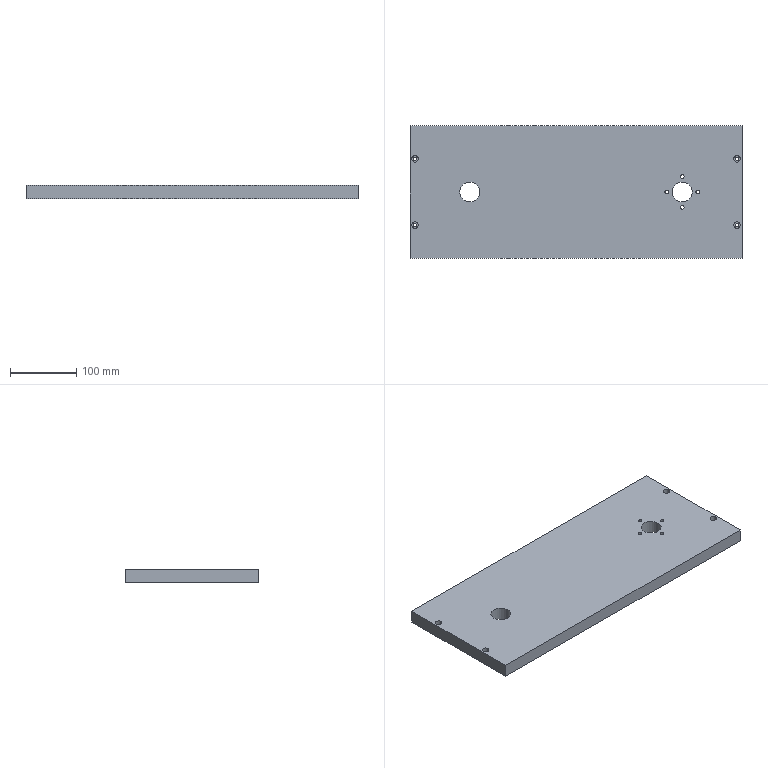Part | NX | features DATUM_CSYS 5, CBORE_HOLE 4, SKETCH 4, EXTRUDE 3, HOLE PACKAGE 1 | 1 solid | 24 faces | box 500 x 200 x 20 mm | volume 1965834 mm3 | cylinder 14 | plane 10 | commonest cylinder face diameters 5.2 x4 5.5 x4 10 x4 30 x2
STEP:
#1=CARTESIAN_POINT('',(183.33,2.75,20.));
#2=VERTEX_POINT('',#1);
#3=CARTESIAN_POINT('',(183.33,0.,20.));
#4=DIRECTION('',(0.,0.,1.));
#5=DIRECTION('',(0.,1.,0.));
#6=AXIS2_PLACEMENT_3D('',#3,#4,#5);
#7=CIRCLE('',#6,2.75);
#8=EDGE_CURVE('',#2,#2,#7,.T.);
#9=ORIENTED_EDGE('',*,*,#8,.F.);
#10=EDGE_LOOP('',(#9));
#11=FACE_BOUND('',#10,.T.);
#12=CARTESIAN_POINT('',(157.25,23.33,20.));
#13=VERTEX_POINT('',#12);
#14=CARTESIAN_POINT('',(160.,23.33,20.));
#15=DIRECTION('',(0.,0.,1.));
#16=DIRECTION('',(-1.,0.,0.));
#17=AXIS2_PLACEMENT_3D('',#14,#15,#16);
#18=CIRCLE('',#17,2.75);
#19=EDGE_CURVE('',#13,#13,#18,.T.);
#20=ORIENTED_EDGE('',*,*,#19,.F.);
#21=EDGE_LOOP('',(#20));
#22=FACE_BOUND('',#21,.T.);
#23=CARTESIAN_POINT('',(162.75,-23.33,20.));
#24=VERTEX_POINT('',#23);
#25=CARTESIAN_POINT('',(160.,-23.33,20.));
#26=DIRECTION('',(0.,0.,1.));
#27=DIRECTION('',(1.,0.,0.));
#28=AXIS2_PLACEMENT_3D('',#25,#26,#27);
#29=CIRCLE('',#28,2.75);
#30=EDGE_CURVE('',#24,#24,#29,.T.);
#31=ORIENTED_EDGE('',*,*,#30,.F.);
#32=EDGE_LOOP('',(#31));
#33=FACE_BOUND('',#32,.T.);
#34=CARTESIAN_POINT('',(136.67,-2.75,20.));
#35=VERTEX_POINT('',#34);
#36=CARTESIAN_POINT('',(136.67,0.,20.));
#37=DIRECTION('',(0.,0.,1.));
#38=DIRECTION('',(0.,-1.,0.));
#39=AXIS2_PLACEMENT_3D('',#36,#37,#38);
#40=CIRCLE('',#39,2.75);
#41=EDGE_CURVE('',#35,#35,#40,.T.);
#42=ORIENTED_EDGE('',*,*,#41,.F.);
#43=EDGE_LOOP('',(#42));
#44=FACE_BOUND('',#43,.T.);
#45=CARTESIAN_POINT('',(237.5,50.,20.));
#46=VERTEX_POINT('',#45);
#47=CARTESIAN_POINT('',(242.5,50.,20.));
#48=DIRECTION('',(0.,0.,-1.));
#49=DIRECTION('',(-1.,0.,0.));
#50=AXIS2_PLACEMENT_3D('',#47,#48,#49);
#51=CIRCLE('',#50,5.);
#52=EDGE_CURVE('',#46,#46,#51,.T.);
#53=ORIENTED_EDGE('',*,*,#52,.T.);
#54=EDGE_LOOP('',(#53));
#55=FACE_BOUND('',#54,.T.);
#56=CARTESIAN_POINT('',(237.5,-50.,20.));
#57=VERTEX_POINT('',#56);
#58=CARTESIAN_POINT('',(242.5,-50.,20.));
#59=DIRECTION('',(0.,0.,-1.));
#60=DIRECTION('',(-1.,0.,0.));
#61=AXIS2_PLACEMENT_3D('',#58,#59,#60);
#62=CIRCLE('',#61,5.);
#63=EDGE_CURVE('',#57,#57,#62,.T.);
#64=ORIENTED_EDGE('',*,*,#63,.T.);
#65=EDGE_LOOP('',(#64));
#66=FACE_BOUND('',#65,.T.);
#67=CARTESIAN_POINT('',(-247.5,50.,20.));
#68=VERTEX_POINT('',#67);
#69=CARTESIAN_POINT('',(-242.5,50.,20.));
#70=DIRECTION('',(0.,0.,-1.));
#71=DIRECTION('',(-1.,0.,0.));
#72=AXIS2_PLACEMENT_3D('',#69,#70,#71);
#73=CIRCLE('',#72,5.);
#74=EDGE_CURVE('',#68,#68,#73,.T.);
#75=ORIENTED_EDGE('',*,*,#74,.T.);
#76=EDGE_LOOP('',(#75));
#77=FACE_BOUND('',#76,.T.);
#78=CARTESIAN_POINT('',(-247.5,-50.,20.));
#79=VERTEX_POINT('',#78);
#80=CARTESIAN_POINT('',(-242.5,-50.,20.));
#81=DIRECTION('',(0.,0.,-1.));
#82=DIRECTION('',(-1.,0.,0.));
#83=AXIS2_PLACEMENT_3D('',#80,#81,#82);
#84=CIRCLE('',#83,5.);
#85=EDGE_CURVE('',#79,#79,#84,.T.);
#86=ORIENTED_EDGE('',*,*,#85,.T.);
#87=EDGE_LOOP('',(#86));
#88=FACE_BOUND('',#87,.T.);
#89=CARTESIAN_POINT('',(-250.,100.,20.));
#90=VERTEX_POINT('',#89);
#91=CARTESIAN_POINT('',(-250.,-100.,20.));
#92=VERTEX_POINT('',#91);
#93=CARTESIAN_POINT('',(-250.,100.,20.));
#94=DIRECTION('',(0.,-1.,0.));
#95=VECTOR('',#94,1000.);
#96=LINE('',#93,#95);
#97=EDGE_CURVE('',#90,#92,#96,.T.);
#98=ORIENTED_EDGE('',*,*,#97,.T.);
#99=CARTESIAN_POINT('',(250.,-100.,20.));
#100=VERTEX_POINT('',#99);
#101=CARTESIAN_POINT('',(-250.,-100.,20.));
#102=DIRECTION('',(1.,0.,0.));
#103=VECTOR('',#102,1000.);
#104=LINE('',#101,#103);
#105=EDGE_CURVE('',#92,#100,#104,.T.);
#106=ORIENTED_EDGE('',*,*,#105,.T.);
#107=CARTESIAN_POINT('',(250.,100.,20.));
#108=VERTEX_POINT('',#107);
#109=CARTESIAN_POINT('',(250.,-100.,20.));
#110=DIRECTION('',(0.,1.,0.));
#111=VECTOR('',#110,1000.);
#112=LINE('',#109,#111);
#113=EDGE_CURVE('',#100,#108,#112,.T.);
#114=ORIENTED_EDGE('',*,*,#113,.T.);
#115=CARTESIAN_POINT('',(250.,100.,20.));
#116=DIRECTION('',(-1.,0.,0.));
#117=VECTOR('',#116,1000.);
#118=LINE('',#115,#117);
#119=EDGE_CURVE('',#108,#90,#118,.T.);
#120=ORIENTED_EDGE('',*,*,#119,.T.);
#121=EDGE_LOOP('',(#98,#106,#114,#120));
#122=FACE_BOUND('',#121,.T.);
#123=CARTESIAN_POINT('',(145.,0.,20.));
#124=VERTEX_POINT('',#123);
#125=CARTESIAN_POINT('',(160.,0.,20.));
#126=DIRECTION('',(0.,0.,-1.));
#127=DIRECTION('',(-1.,0.,0.));
#128=AXIS2_PLACEMENT_3D('',#125,#126,#127);
#129=CIRCLE('',#128,15.);
#130=EDGE_CURVE('',#124,#124,#129,.T.);
#131=ORIENTED_EDGE('',*,*,#130,.T.);
#132=EDGE_LOOP('',(#131));
#133=FACE_BOUND('',#132,.T.);
#134=CARTESIAN_POINT('',(-145.,0.,20.));
#135=VERTEX_POINT('',#134);
#136=CARTESIAN_POINT('',(-160.,0.,20.));
#137=DIRECTION('',(0.,0.,1.));
#138=DIRECTION('',(1.,0.,0.));
#139=AXIS2_PLACEMENT_3D('',#136,#137,#138);
#140=CIRCLE('',#139,15.);
#141=EDGE_CURVE('',#135,#135,#140,.T.);
#142=ORIENTED_EDGE('',*,*,#141,.F.);
#143=EDGE_LOOP('',(#142));
#144=FACE_BOUND('',#143,.T.);
#145=CARTESIAN_POINT('',(0.,0.,20.));
#146=DIRECTION('',(0.,0.,1.));
#147=DIRECTION('',(1.,0.,0.));
#148=AXIS2_PLACEMENT_3D('',#145,#146,#147);
#149=PLANE('',#148);
#150=ADVANCED_FACE('',(#11,#22,#33,#44,#55,#66,#77,#88,#122,#133,#144),#149,.T.);
#151=CARTESIAN_POINT('',(186.08,0.,0.));
#152=VERTEX_POINT('',#151);
#153=CARTESIAN_POINT('',(183.33,0.,0.));
#154=DIRECTION('',(0.,0.,1.));
#155=DIRECTION('',(1.,0.,0.));
#156=AXIS2_PLACEMENT_3D('',#153,#154,#155);
#157=CIRCLE('',#156,2.75);
#158=EDGE_CURVE('',#152,#152,#157,.T.);
#159=ORIENTED_EDGE('',*,*,#158,.T.);
#160=EDGE_LOOP('',(#159));
#161=FACE_BOUND('',#160,.T.);
#162=CARTESIAN_POINT('',(162.75,23.33,0.));
#163=VERTEX_POINT('',#162);
#164=CARTESIAN_POINT('',(160.,23.33,0.));
#165=DIRECTION('',(0.,0.,1.));
#166=DIRECTION('',(1.,0.,0.));
#167=AXIS2_PLACEMENT_3D('',#164,#165,#166);
#168=CIRCLE('',#167,2.75);
#169=EDGE_CURVE('',#163,#163,#168,.T.);
#170=ORIENTED_EDGE('',*,*,#169,.T.);
#171=EDGE_LOOP('',(#170));
#172=FACE_BOUND('',#171,.T.);
#173=CARTESIAN_POINT('',(162.75,-23.33,0.));
#174=VERTEX_POINT('',#173);
#175=CARTESIAN_POINT('',(160.,-23.33,0.));
#176=DIRECTION('',(0.,0.,1.));
#177=DIRECTION('',(1.,0.,0.));
#178=AXIS2_PLACEMENT_3D('',#175,#176,#177);
#179=CIRCLE('',#178,2.75);
#180=EDGE_CURVE('',#174,#174,#179,.T.);
#181=ORIENTED_EDGE('',*,*,#180,.T.);
#182=EDGE_LOOP('',(#181));
#183=FACE_BOUND('',#182,.T.);
#184=CARTESIAN_POINT('',(139.42,0.,0.));
#185=VERTEX_POINT('',#184);
#186=CARTESIAN_POINT('',(136.67,0.,0.));
#187=DIRECTION('',(0.,0.,1.));
#188=DIRECTION('',(1.,0.,0.));
#189=AXIS2_PLACEMENT_3D('',#186,#187,#188);
#190=CIRCLE('',#189,2.75);
#191=EDGE_CURVE('',#185,#185,#190,.T.);
#192=ORIENTED_EDGE('',*,*,#191,.T.);
#193=EDGE_LOOP('',(#192));
#194=FACE_BOUND('',#193,.T.);
#195=CARTESIAN_POINT('',(245.1,50.,0.));
#196=VERTEX_POINT('',#195);
#197=CARTESIAN_POINT('',(242.5,50.,0.));
#198=DIRECTION('',(0.,0.,1.));
#199=DIRECTION('',(1.,0.,0.));
#200=AXIS2_PLACEMENT_3D('',#197,#198,#199);
#201=CIRCLE('',#200,2.6);
#202=EDGE_CURVE('',#196,#196,#201,.T.);
#203=ORIENTED_EDGE('',*,*,#202,.T.);
#204=EDGE_LOOP('',(#203));
#205=FACE_BOUND('',#204,.T.);
#206=CARTESIAN_POINT('',(245.1,-50.,0.));
#207=VERTEX_POINT('',#206);
#208=CARTESIAN_POINT('',(242.5,-50.,0.));
#209=DIRECTION('',(0.,0.,1.));
#210=DIRECTION('',(1.,0.,0.));
#211=AXIS2_PLACEMENT_3D('',#208,#209,#210);
#212=CIRCLE('',#211,2.6);
#213=EDGE_CURVE('',#207,#207,#212,.T.);
#214=ORIENTED_EDGE('',*,*,#213,.T.);
#215=EDGE_LOOP('',(#214));
#216=FACE_BOUND('',#215,.T.);
#217=CARTESIAN_POINT('',(-239.9,50.,0.));
#218=VERTEX_POINT('',#217);
#219=CARTESIAN_POINT('',(-242.5,50.,0.));
#220=DIRECTION('',(0.,0.,1.));
#221=DIRECTION('',(1.,0.,0.));
#222=AXIS2_PLACEMENT_3D('',#219,#220,#221);
#223=CIRCLE('',#222,2.6);
#224=EDGE_CURVE('',#218,#218,#223,.T.);
#225=ORIENTED_EDGE('',*,*,#224,.T.);
#226=EDGE_LOOP('',(#225));
#227=FACE_BOUND('',#226,.T.);
#228=CARTESIAN_POINT('',(-239.9,-50.,0.));
#229=VERTEX_POINT('',#228);
#230=CARTESIAN_POINT('',(-242.5,-50.,0.));
#231=DIRECTION('',(0.,0.,1.));
#232=DIRECTION('',(1.,0.,0.));
#233=AXIS2_PLACEMENT_3D('',#230,#231,#232);
#234=CIRCLE('',#233,2.6);
#235=EDGE_CURVE('',#229,#229,#234,.T.);
#236=ORIENTED_EDGE('',*,*,#235,.T.);
#237=EDGE_LOOP('',(#236));
#238=FACE_BOUND('',#237,.T.);
#239=CARTESIAN_POINT('',(145.,0.,0.));
#240=VERTEX_POINT('',#239);
#241=CARTESIAN_POINT('',(160.,0.,0.));
#242=DIRECTION('',(0.,0.,-1.));
#243=DIRECTION('',(-1.,0.,0.));
#244=AXIS2_PLACEMENT_3D('',#241,#242,#243);
#245=CIRCLE('',#244,15.);
#246=EDGE_CURVE('',#240,#240,#245,.T.);
#247=ORIENTED_EDGE('',*,*,#246,.F.);
#248=EDGE_LOOP('',(#247));
#249=FACE_BOUND('',#248,.T.);
#250=CARTESIAN_POINT('',(-250.,100.,0.));
#251=VERTEX_POINT('',#250);
#252=CARTESIAN_POINT('',(-250.,-100.,0.));
#253=VERTEX_POINT('',#252);
#254=CARTESIAN_POINT('',(-250.,100.,0.));
#255=DIRECTION('',(0.,-1.,0.));
#256=VECTOR('',#255,1000.);
#257=LINE('',#254,#256);
#258=EDGE_CURVE('',#251,#253,#257,.T.);
#259=ORIENTED_EDGE('',*,*,#258,.F.);
#260=CARTESIAN_POINT('',(250.,100.,0.));
#261=VERTEX_POINT('',#260);
#262=CARTESIAN_POINT('',(250.,100.,0.));
#263=DIRECTION('',(-1.,0.,0.));
#264=VECTOR('',#263,1000.);
#265=LINE('',#262,#264);
#266=EDGE_CURVE('',#261,#251,#265,.T.);
#267=ORIENTED_EDGE('',*,*,#266,.F.);
#268=CARTESIAN_POINT('',(250.,-100.,0.));
#269=VERTEX_POINT('',#268);
#270=CARTESIAN_POINT('',(250.,-100.,0.));
#271=DIRECTION('',(0.,1.,0.));
#272=VECTOR('',#271,1000.);
#273=LINE('',#270,#272);
#274=EDGE_CURVE('',#269,#261,#273,.T.);
#275=ORIENTED_EDGE('',*,*,#274,.F.);
#276=CARTESIAN_POINT('',(-250.,-100.,0.));
#277=DIRECTION('',(1.,0.,0.));
#278=VECTOR('',#277,1000.);
#279=LINE('',#276,#278);
#280=EDGE_CURVE('',#253,#269,#279,.T.);
#281=ORIENTED_EDGE('',*,*,#280,.F.);
#282=EDGE_LOOP('',(#259,#267,#275,#281));
#283=FACE_BOUND('',#282,.T.);
#284=CARTESIAN_POINT('',(-145.,0.,0.));
#285=VERTEX_POINT('',#284);
#286=CARTESIAN_POINT('',(-160.,0.,0.));
#287=DIRECTION('',(0.,0.,1.));
#288=DIRECTION('',(1.,0.,0.));
#289=AXIS2_PLACEMENT_3D('',#286,#287,#288);
#290=CIRCLE('',#289,15.);
#291=EDGE_CURVE('',#285,#285,#290,.T.);
#292=ORIENTED_EDGE('',*,*,#291,.T.);
#293=EDGE_LOOP('',(#292));
#294=FACE_BOUND('',#293,.T.);
#295=CARTESIAN_POINT('',(0.,0.,0.));
#296=DIRECTION('',(0.,0.,1.));
#297=DIRECTION('',(1.,0.,0.));
#298=AXIS2_PLACEMENT_3D('',#295,#296,#297);
#299=PLANE('',#298);
#300=ADVANCED_FACE('',(#161,#172,#183,#194,#205,#216,#227,#238,#249,#283,#294),#299,.F.);
#301=ORIENTED_EDGE('',*,*,#258,.T.);
#302=CARTESIAN_POINT('',(-250.,-100.,20.));
#303=DIRECTION('',(0.,0.,-1.));
#304=VECTOR('',#303,1000.);
#305=LINE('',#302,#304);
#306=EDGE_CURVE('',#92,#253,#305,.T.);
#307=ORIENTED_EDGE('',*,*,#306,.F.);
#308=ORIENTED_EDGE('',*,*,#97,.F.);
#309=CARTESIAN_POINT('',(-250.,100.,20.));
#310=DIRECTION('',(0.,0.,-1.));
#311=VECTOR('',#310,1000.);
#312=LINE('',#309,#311);
#313=EDGE_CURVE('',#90,#251,#312,.T.);
#314=ORIENTED_EDGE('',*,*,#313,.T.);
#315=EDGE_LOOP('',(#301,#307,#308,#314));
#316=FACE_BOUND('',#315,.T.);
#317=CARTESIAN_POINT('',(-250.,100.,20.));
#318=DIRECTION('',(1.,0.,0.));
#319=DIRECTION('',(0.,1.,0.));
#320=AXIS2_PLACEMENT_3D('',#317,#318,#319);
#321=PLANE('',#320);
#322=ADVANCED_FACE('',(#316),#321,.F.);
#323=ORIENTED_EDGE('',*,*,#280,.T.);
#324=CARTESIAN_POINT('',(250.,-100.,20.));
#325=DIRECTION('',(0.,0.,-1.));
#326=VECTOR('',#325,1000.);
#327=LINE('',#324,#326);
#328=EDGE_CURVE('',#100,#269,#327,.T.);
#329=ORIENTED_EDGE('',*,*,#328,.F.);
#330=ORIENTED_EDGE('',*,*,#105,.F.);
#331=ORIENTED_EDGE('',*,*,#306,.T.);
#332=EDGE_LOOP('',(#323,#329,#330,#331));
#333=FACE_BOUND('',#332,.T.);
#334=CARTESIAN_POINT('',(-250.,-100.,20.));
#335=DIRECTION('',(0.,1.,0.));
#336=DIRECTION('',(0.,0.,1.));
#337=AXIS2_PLACEMENT_3D('',#334,#335,#336);
#338=PLANE('',#337);
#339=ADVANCED_FACE('',(#333),#338,.F.);
#340=ORIENTED_EDGE('',*,*,#274,.T.);
#341=CARTESIAN_POINT('',(250.,100.,20.));
#342=DIRECTION('',(0.,0.,-1.));
#343=VECTOR('',#342,1000.);
#344=LINE('',#341,#343);
#345=EDGE_CURVE('',#108,#261,#344,.T.);
#346=ORIENTED_EDGE('',*,*,#345,.F.);
#347=ORIENTED_EDGE('',*,*,#113,.F.);
#348=ORIENTED_EDGE('',*,*,#328,.T.);
#349=EDGE_LOOP('',(#340,#346,#347,#348));
#350=FACE_BOUND('',#349,.T.);
#351=CARTESIAN_POINT('',(250.,-100.,20.));
#352=DIRECTION('',(-1.,0.,0.));
#353=DIRECTION('',(0.,-1.,0.));
#354=AXIS2_PLACEMENT_3D('',#351,#352,#353);
#355=PLANE('',#354);
#356=ADVANCED_FACE('',(#350),#355,.F.);
#357=ORIENTED_EDGE('',*,*,#266,.T.);
#358=ORIENTED_EDGE('',*,*,#313,.F.);
#359=ORIENTED_EDGE('',*,*,#119,.F.);
#360=ORIENTED_EDGE('',*,*,#345,.T.);
#361=EDGE_LOOP('',(#357,#358,#359,#360));
#362=FACE_BOUND('',#361,.T.);
#363=CARTESIAN_POINT('',(250.,100.,20.));
#364=DIRECTION('',(0.,-1.,0.));
#365=DIRECTION('',(0.,0.,-1.));
#366=AXIS2_PLACEMENT_3D('',#363,#364,#365);
#367=PLANE('',#366);
#368=ADVANCED_FACE('',(#362),#367,.F.);
#369=ORIENTED_EDGE('',*,*,#130,.F.);
#370=EDGE_LOOP('',(#369));
#371=FACE_BOUND('',#370,.T.);
#372=ORIENTED_EDGE('',*,*,#246,.T.);
#373=EDGE_LOOP('',(#372));
#374=FACE_BOUND('',#373,.T.);
#375=CARTESIAN_POINT('',(160.,0.,20.));
#376=DIRECTION('',(0.,0.,-1.));
#377=DIRECTION('',(-1.,0.,0.));
#378=AXIS2_PLACEMENT_3D('',#375,#376,#377);
#379=CYLINDRICAL_SURFACE('',#378,15.);
#380=ADVANCED_FACE('',(#371,#374),#379,.F.);
#381=ORIENTED_EDGE('',*,*,#141,.T.);
#382=EDGE_LOOP('',(#381));
#383=FACE_BOUND('',#382,.T.);
#384=ORIENTED_EDGE('',*,*,#291,.F.);
#385=EDGE_LOOP('',(#384));
#386=FACE_BOUND('',#385,.T.);
#387=CARTESIAN_POINT('',(-160.,0.,20.));
#388=DIRECTION('',(0.,0.,-1.));
#389=DIRECTION('',(-1.,0.,0.));
#390=AXIS2_PLACEMENT_3D('',#387,#388,#389);
#391=CYLINDRICAL_SURFACE('',#390,15.);
#392=ADVANCED_FACE('',(#383,#386),#391,.F.);
#393=CARTESIAN_POINT('',(-245.1,-50.,10.));
#394=VERTEX_POINT('',#393);
#395=CARTESIAN_POINT('',(-242.5,-50.,10.));
#396=DIRECTION('',(0.,0.,-1.));
#397=DIRECTION('',(-1.,0.,0.));
#398=AXIS2_PLACEMENT_3D('',#395,#396,#397);
#399=CIRCLE('',#398,2.6);
#400=EDGE_CURVE('',#394,#394,#399,.F.);
#401=ORIENTED_EDGE('',*,*,#400,.T.);
#402=EDGE_LOOP('',(#401));
#403=FACE_BOUND('',#402,.T.);
#404=ORIENTED_EDGE('',*,*,#235,.F.);
#405=EDGE_LOOP('',(#404));
#406=FACE_BOUND('',#405,.T.);
#407=CARTESIAN_POINT('',(-242.5,-50.,-30.));
#408=DIRECTION('',(0.,0.,-1.));
#409=DIRECTION('',(-1.,0.,0.));
#410=AXIS2_PLACEMENT_3D('',#407,#408,#409);
#411=CYLINDRICAL_SURFACE('',#410,2.6);
#412=ADVANCED_FACE('',(#403,#406),#411,.F.);
#413=ORIENTED_EDGE('',*,*,#400,.F.);
#414=EDGE_LOOP('',(#413));
#415=FACE_BOUND('',#414,.T.);
#416=CARTESIAN_POINT('',(-247.5,-50.,10.));
#417=VERTEX_POINT('',#416);
#418=CARTESIAN_POINT('',(-242.5,-50.,10.));
#419=DIRECTION('',(0.,0.,-1.));
#420=DIRECTION('',(-1.,0.,0.));
#421=AXIS2_PLACEMENT_3D('',#418,#419,#420);
#422=CIRCLE('',#421,5.);
#423=EDGE_CURVE('',#417,#417,#422,.F.);
#424=ORIENTED_EDGE('',*,*,#423,.T.);
#425=EDGE_LOOP('',(#424));
#426=FACE_BOUND('',#425,.T.);
#427=CARTESIAN_POINT('',(-242.5,-50.,10.));
#428=DIRECTION('',(0.,0.,-1.));
#429=DIRECTION('',(-1.,0.,0.));
#430=AXIS2_PLACEMENT_3D('',#427,#428,#429);
#431=PLANE('',#430);
#432=ADVANCED_FACE('',(#415,#426),#431,.F.);
#433=ORIENTED_EDGE('',*,*,#423,.F.);
#434=EDGE_LOOP('',(#433));
#435=FACE_BOUND('',#434,.T.);
#436=ORIENTED_EDGE('',*,*,#85,.F.);
#437=EDGE_LOOP('',(#436));
#438=FACE_BOUND('',#437,.T.);
#439=CARTESIAN_POINT('',(-242.5,-50.,20.));
#440=DIRECTION('',(0.,0.,-1.));
#441=DIRECTION('',(-1.,0.,0.));
#442=AXIS2_PLACEMENT_3D('',#439,#440,#441);
#443=CYLINDRICAL_SURFACE('',#442,5.);
#444=ADVANCED_FACE('',(#435,#438),#443,.F.);
#445=CARTESIAN_POINT('',(-245.1,50.,10.));
#446=VERTEX_POINT('',#445);
#447=CARTESIAN_POINT('',(-242.5,50.,10.));
#448=DIRECTION('',(0.,0.,-1.));
#449=DIRECTION('',(-1.,0.,0.));
#450=AXIS2_PLACEMENT_3D('',#447,#448,#449);
#451=CIRCLE('',#450,2.6);
#452=EDGE_CURVE('',#446,#446,#451,.F.);
#453=ORIENTED_EDGE('',*,*,#452,.T.);
#454=EDGE_LOOP('',(#453));
#455=FACE_BOUND('',#454,.T.);
#456=ORIENTED_EDGE('',*,*,#224,.F.);
#457=EDGE_LOOP('',(#456));
#458=FACE_BOUND('',#457,.T.);
#459=CARTESIAN_POINT('',(-242.5,50.,-30.));
#460=DIRECTION('',(0.,0.,-1.));
#461=DIRECTION('',(-1.,0.,0.));
#462=AXIS2_PLACEMENT_3D('',#459,#460,#461);
#463=CYLINDRICAL_SURFACE('',#462,2.6);
#464=ADVANCED_FACE('',(#455,#458),#463,.F.);
#465=ORIENTED_EDGE('',*,*,#452,.F.);
#466=EDGE_LOOP('',(#465));
#467=FACE_BOUND('',#466,.T.);
#468=CARTESIAN_POINT('',(-247.5,50.,10.));
#469=VERTEX_POINT('',#468);
#470=CARTESIAN_POINT('',(-242.5,50.,10.));
#471=DIRECTION('',(0.,0.,-1.));
#472=DIRECTION('',(-1.,0.,0.));
#473=AXIS2_PLACEMENT_3D('',#470,#471,#472);
#474=CIRCLE('',#473,5.);
#475=EDGE_CURVE('',#469,#469,#474,.F.);
#476=ORIENTED_EDGE('',*,*,#475,.T.);
#477=EDGE_LOOP('',(#476));
#478=FACE_BOUND('',#477,.T.);
#479=CARTESIAN_POINT('',(-242.5,50.,10.));
#480=DIRECTION('',(0.,0.,-1.));
#481=DIRECTION('',(-1.,0.,0.));
#482=AXIS2_PLACEMENT_3D('',#479,#480,#481);
#483=PLANE('',#482);
#484=ADVANCED_FACE('',(#467,#478),#483,.F.);
#485=ORIENTED_EDGE('',*,*,#475,.F.);
#486=EDGE_LOOP('',(#485));
#487=FACE_BOUND('',#486,.T.);
#488=ORIENTED_EDGE('',*,*,#74,.F.);
#489=EDGE_LOOP('',(#488));
#490=FACE_BOUND('',#489,.T.);
#491=CARTESIAN_POINT('',(-242.5,50.,20.));
#492=DIRECTION('',(0.,0.,-1.));
#493=DIRECTION('',(-1.,0.,0.));
#494=AXIS2_PLACEMENT_3D('',#491,#492,#493);
#495=CYLINDRICAL_SURFACE('',#494,5.);
#496=ADVANCED_FACE('',(#487,#490),#495,.F.);
#497=CARTESIAN_POINT('',(239.9,-50.,10.));
#498=VERTEX_POINT('',#497);
#499=CARTESIAN_POINT('',(242.5,-50.,10.));
#500=DIRECTION('',(0.,0.,-1.));
#501=DIRECTION('',(-1.,0.,0.));
#502=AXIS2_PLACEMENT_3D('',#499,#500,#501);
#503=CIRCLE('',#502,2.6);
#504=EDGE_CURVE('',#498,#498,#503,.F.);
#505=ORIENTED_EDGE('',*,*,#504,.T.);
#506=EDGE_LOOP('',(#505));
#507=FACE_BOUND('',#506,.T.);
#508=ORIENTED_EDGE('',*,*,#213,.F.);
#509=EDGE_LOOP('',(#508));
#510=FACE_BOUND('',#509,.T.);
#511=CARTESIAN_POINT('',(242.5,-50.,-30.));
#512=DIRECTION('',(0.,0.,-1.));
#513=DIRECTION('',(-1.,0.,0.));
#514=AXIS2_PLACEMENT_3D('',#511,#512,#513);
#515=CYLINDRICAL_SURFACE('',#514,2.6);
#516=ADVANCED_FACE('',(#507,#510),#515,.F.);
#517=ORIENTED_EDGE('',*,*,#504,.F.);
#518=EDGE_LOOP('',(#517));
#519=FACE_BOUND('',#518,.T.);
#520=CARTESIAN_POINT('',(237.5,-50.,10.));
#521=VERTEX_POINT('',#520);
#522=CARTESIAN_POINT('',(242.5,-50.,10.));
#523=DIRECTION('',(0.,0.,-1.));
#524=DIRECTION('',(-1.,0.,0.));
#525=AXIS2_PLACEMENT_3D('',#522,#523,#524);
#526=CIRCLE('',#525,5.);
#527=EDGE_CURVE('',#521,#521,#526,.F.);
#528=ORIENTED_EDGE('',*,*,#527,.T.);
#529=EDGE_LOOP('',(#528));
#530=FACE_BOUND('',#529,.T.);
#531=CARTESIAN_POINT('',(242.5,-50.,10.));
#532=DIRECTION('',(0.,0.,-1.));
#533=DIRECTION('',(-1.,0.,0.));
#534=AXIS2_PLACEMENT_3D('',#531,#532,#533);
#535=PLANE('',#534);
#536=ADVANCED_FACE('',(#519,#530),#535,.F.);
#537=ORIENTED_EDGE('',*,*,#527,.F.);
#538=EDGE_LOOP('',(#537));
#539=FACE_BOUND('',#538,.T.);
#540=ORIENTED_EDGE('',*,*,#63,.F.);
#541=EDGE_LOOP('',(#540));
#542=FACE_BOUND('',#541,.T.);
#543=CARTESIAN_POINT('',(242.5,-50.,20.));
#544=DIRECTION('',(0.,0.,-1.));
#545=DIRECTION('',(-1.,0.,0.));
#546=AXIS2_PLACEMENT_3D('',#543,#544,#545);
#547=CYLINDRICAL_SURFACE('',#546,5.);
#548=ADVANCED_FACE('',(#539,#542),#547,.F.);
#549=CARTESIAN_POINT('',(239.9,50.,10.));
#550=VERTEX_POINT('',#549);
#551=CARTESIAN_POINT('',(242.5,50.,10.));
#552=DIRECTION('',(0.,0.,-1.));
#553=DIRECTION('',(-1.,0.,0.));
#554=AXIS2_PLACEMENT_3D('',#551,#552,#553);
#555=CIRCLE('',#554,2.6);
#556=EDGE_CURVE('',#550,#550,#555,.F.);
#557=ORIENTED_EDGE('',*,*,#556,.T.);
#558=EDGE_LOOP('',(#557));
#559=FACE_BOUND('',#558,.T.);
#560=ORIENTED_EDGE('',*,*,#202,.F.);
#561=EDGE_LOOP('',(#560));
#562=FACE_BOUND('',#561,.T.);
#563=CARTESIAN_POINT('',(242.5,50.,-30.));
#564=DIRECTION('',(0.,0.,-1.));
#565=DIRECTION('',(-1.,0.,0.));
#566=AXIS2_PLACEMENT_3D('',#563,#564,#565);
#567=CYLINDRICAL_SURFACE('',#566,2.6);
#568=ADVANCED_FACE('',(#559,#562),#567,.F.);
#569=ORIENTED_EDGE('',*,*,#556,.F.);
#570=EDGE_LOOP('',(#569));
#571=FACE_BOUND('',#570,.T.);
#572=CARTESIAN_POINT('',(237.5,50.,10.));
#573=VERTEX_POINT('',#572);
#574=CARTESIAN_POINT('',(242.5,50.,10.));
#575=DIRECTION('',(0.,0.,-1.));
#576=DIRECTION('',(-1.,0.,0.));
#577=AXIS2_PLACEMENT_3D('',#574,#575,#576);
#578=CIRCLE('',#577,5.);
#579=EDGE_CURVE('',#573,#573,#578,.F.);
#580=ORIENTED_EDGE('',*,*,#579,.T.);
#581=EDGE_LOOP('',(#580));
#582=FACE_BOUND('',#581,.T.);
#583=CARTESIAN_POINT('',(242.5,50.,10.));
#584=DIRECTION('',(0.,0.,-1.));
#585=DIRECTION('',(-1.,0.,0.));
#586=AXIS2_PLACEMENT_3D('',#583,#584,#585);
#587=PLANE('',#586);
#588=ADVANCED_FACE('',(#571,#582),#587,.F.);
#589=ORIENTED_EDGE('',*,*,#579,.F.);
#590=EDGE_LOOP('',(#589));
#591=FACE_BOUND('',#590,.T.);
#592=ORIENTED_EDGE('',*,*,#52,.F.);
#593=EDGE_LOOP('',(#592));
#594=FACE_BOUND('',#593,.T.);
#595=CARTESIAN_POINT('',(242.5,50.,20.));
#596=DIRECTION('',(0.,0.,-1.));
#597=DIRECTION('',(-1.,0.,0.));
#598=AXIS2_PLACEMENT_3D('',#595,#596,#597);
#599=CYLINDRICAL_SURFACE('',#598,5.);
#600=ADVANCED_FACE('',(#591,#594),#599,.F.);
#601=ORIENTED_EDGE('',*,*,#41,.T.);
#602=EDGE_LOOP('',(#601));
#603=FACE_BOUND('',#602,.T.);
#604=ORIENTED_EDGE('',*,*,#191,.F.);
#605=EDGE_LOOP('',(#604));
#606=FACE_BOUND('',#605,.T.);
#607=CARTESIAN_POINT('',(136.67,0.,-35.));
#608=DIRECTION('',(0.,0.,1.));
#609=DIRECTION('',(1.,0.,0.));
#610=AXIS2_PLACEMENT_3D('',#607,#608,#609);
#611=CYLINDRICAL_SURFACE('',#610,2.75);
#612=ADVANCED_FACE('',(#603,#606),#611,.F.);
#613=ORIENTED_EDGE('',*,*,#30,.T.);
#614=EDGE_LOOP('',(#613));
#615=FACE_BOUND('',#614,.T.);
#616=ORIENTED_EDGE('',*,*,#180,.F.);
#617=EDGE_LOOP('',(#616));
#618=FACE_BOUND('',#617,.T.);
#619=CARTESIAN_POINT('',(160.,-23.33,-35.));
#620=DIRECTION('',(0.,0.,1.));
#621=DIRECTION('',(1.,0.,0.));
#622=AXIS2_PLACEMENT_3D('',#619,#620,#621);
#623=CYLINDRICAL_SURFACE('',#622,2.75);
#624=ADVANCED_FACE('',(#615,#618),#623,.F.);
#625=ORIENTED_EDGE('',*,*,#19,.T.);
#626=EDGE_LOOP('',(#625));
#627=FACE_BOUND('',#626,.T.);
#628=ORIENTED_EDGE('',*,*,#169,.F.);
#629=EDGE_LOOP('',(#628));
#630=FACE_BOUND('',#629,.T.);
#631=CARTESIAN_POINT('',(160.,23.33,-35.));
#632=DIRECTION('',(0.,0.,1.));
#633=DIRECTION('',(1.,0.,0.));
#634=AXIS2_PLACEMENT_3D('',#631,#632,#633);
#635=CYLINDRICAL_SURFACE('',#634,2.75);
#636=ADVANCED_FACE('',(#627,#630),#635,.F.);
#637=ORIENTED_EDGE('',*,*,#8,.T.);
#638=EDGE_LOOP('',(#637));
#639=FACE_BOUND('',#638,.T.);
#640=ORIENTED_EDGE('',*,*,#158,.F.);
#641=EDGE_LOOP('',(#640));
#642=FACE_BOUND('',#641,.T.);
#643=CARTESIAN_POINT('',(183.33,0.,-35.));
#644=DIRECTION('',(0.,0.,1.));
#645=DIRECTION('',(1.,0.,0.));
#646=AXIS2_PLACEMENT_3D('',#643,#644,#645);
#647=CYLINDRICAL_SURFACE('',#646,2.75);
#648=ADVANCED_FACE('',(#639,#642),#647,.F.);
#649=CLOSED_SHELL('',(#150,#300,#322,#339,#356,#368,#380,#392,#412,#432,#444,#464,#484,#496,#516,#536,#548,#568,#588,#600,#612,#624,#636,#648));
#650=MANIFOLD_SOLID_BREP('',#649);
#651=(LENGTH_UNIT()NAMED_UNIT(*)SI_UNIT(.MILLI.,.METRE.));
#652=UNCERTAINTY_MEASURE_WITH_UNIT(LENGTH_MEASURE(0.00001),#651,'','');
#653=(NAMED_UNIT(*)PLANE_ANGLE_UNIT()SI_UNIT($,.RADIAN.));
#654=(NAMED_UNIT(*)SI_UNIT($,.STERADIAN.)SOLID_ANGLE_UNIT());
#655=(GEOMETRIC_REPRESENTATION_CONTEXT(3)GLOBAL_UNCERTAINTY_ASSIGNED_CONTEXT((#652))GLOBAL_UNIT_ASSIGNED_CONTEXT((#651,#653,#654))REPRESENTATION_CONTEXT('',''));
#656=ADVANCED_BREP_SHAPE_REPRESENTATION('',(#650),#655);